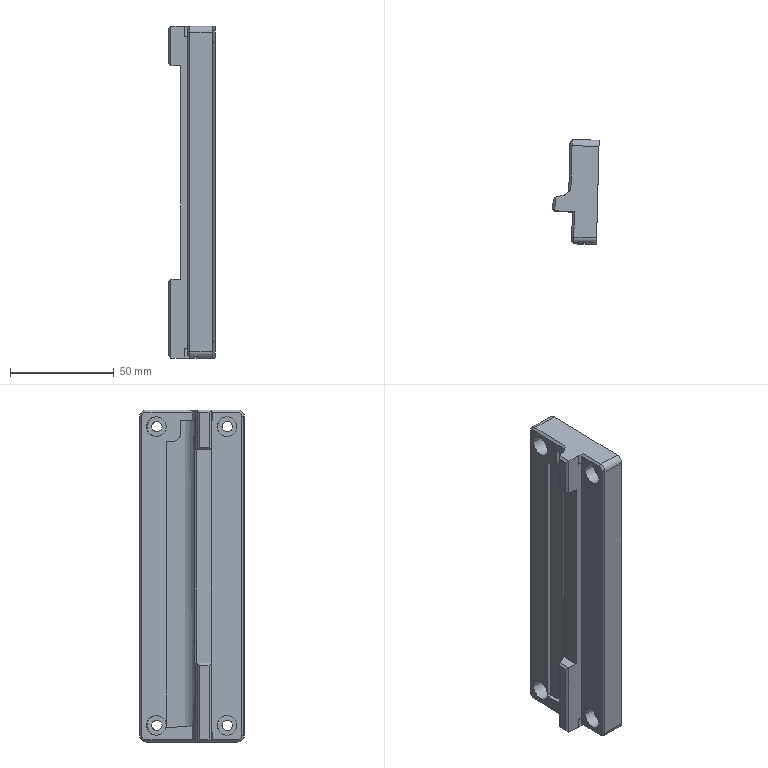Part | STEP file | 222 | 1 solid | 75 faces | box 22.319 x 50.323 x 160 mm | volume 105919 mm3 | plane 44 | cylinder 25 | cone 4 | other 2 | commonest cylinder face diameters 5.11 x8 9.5 x8 6 x5 0.269 x1 0.807 x1 1.526 x1